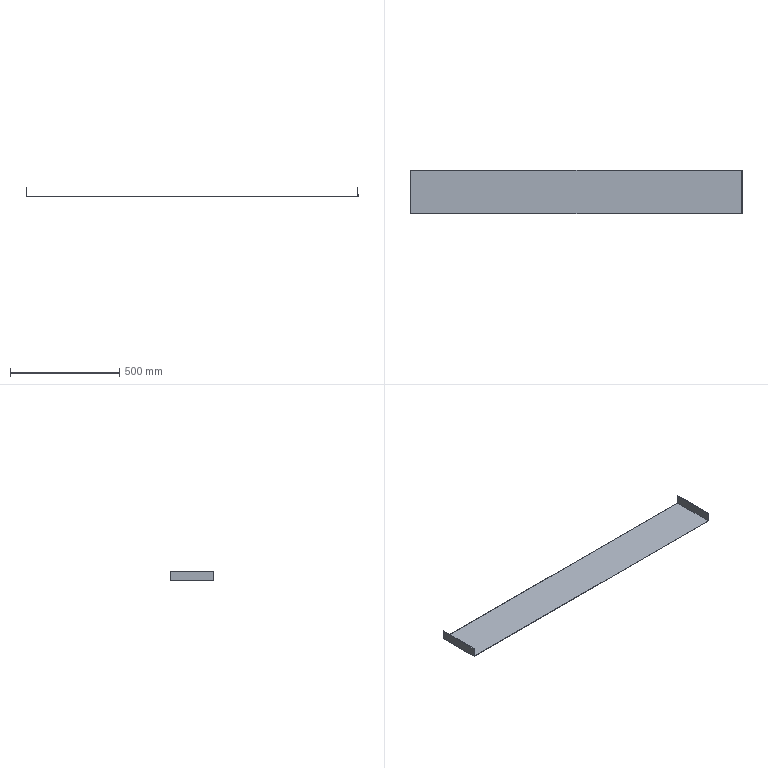Part | SolidWorks | features Extrusion 1, ICE 1, MirrorPattern 1 | 1 solid | 10 faces | box 1518 x 200 x 41 mm | volume 351600 mm3 | plane 10
STEP:
#1=CARTESIAN_POINT('',(-756.,-100.,1.));
#2=VERTEX_POINT('',#1);
#3=CARTESIAN_POINT('',(756.,-100.,1.));
#4=VERTEX_POINT('',#3);
#5=CARTESIAN_POINT('',(-759.,-100.,1.));
#6=DIRECTION('',(1.,0.,0.));
#7=VECTOR('',#6,1000.);
#8=LINE('',#5,#7);
#9=EDGE_CURVE('',#2,#4,#8,.T.);
#10=ORIENTED_EDGE('',*,*,#9,.T.);
#11=CARTESIAN_POINT('',(756.,100.,1.));
#12=VERTEX_POINT('',#11);
#13=CARTESIAN_POINT('',(756.,100.,1.));
#14=DIRECTION('',(0.,1.,0.));
#15=VECTOR('',#14,1000.);
#16=LINE('',#13,#15);
#17=EDGE_CURVE('',#4,#12,#16,.T.);
#18=ORIENTED_EDGE('',*,*,#17,.T.);
#19=CARTESIAN_POINT('',(-756.,100.,1.));
#20=VERTEX_POINT('',#19);
#21=CARTESIAN_POINT('',(-759.,100.,1.));
#22=DIRECTION('',(-1.,0.,0.));
#23=VECTOR('',#22,1000.);
#24=LINE('',#21,#23);
#25=EDGE_CURVE('',#12,#20,#24,.T.);
#26=ORIENTED_EDGE('',*,*,#25,.T.);
#27=CARTESIAN_POINT('',(-756.,100.,1.));
#28=DIRECTION('',(0.,1.,0.));
#29=VECTOR('',#28,1000.);
#30=LINE('',#27,#29);
#31=EDGE_CURVE('',#2,#20,#30,.T.);
#32=ORIENTED_EDGE('',*,*,#31,.F.);
#33=EDGE_LOOP('',(#10,#18,#26,#32));
#34=FACE_OUTER_BOUND('',#33,.T.);
#35=CARTESIAN_POINT('',(0.,0.,1.));
#36=DIRECTION('',(0.,0.,-1.));
#37=DIRECTION('',(-1.,0.,0.));
#38=AXIS2_PLACEMENT_3D('',#35,#36,#37);
#39=PLANE('',#38);
#40=ADVANCED_FACE('',(#34),#39,.F.);
#41=CARTESIAN_POINT('',(759.,-100.,0.));
#42=VERTEX_POINT('',#41);
#43=CARTESIAN_POINT('',(759.,100.,0.));
#44=VERTEX_POINT('',#43);
#45=CARTESIAN_POINT('',(759.,-100.,0.));
#46=DIRECTION('',(0.,1.,0.));
#47=VECTOR('',#46,1000.);
#48=LINE('',#45,#47);
#49=EDGE_CURVE('',#42,#44,#48,.T.);
#50=ORIENTED_EDGE('',*,*,#49,.T.);
#51=CARTESIAN_POINT('',(759.,100.,41.));
#52=VERTEX_POINT('',#51);
#53=CARTESIAN_POINT('',(759.,100.,1.));
#54=DIRECTION('',(0.,0.,-1.));
#55=VECTOR('',#54,1000.);
#56=LINE('',#53,#55);
#57=EDGE_CURVE('',#52,#44,#56,.T.);
#58=ORIENTED_EDGE('',*,*,#57,.F.);
#59=CARTESIAN_POINT('',(759.,-100.,41.));
#60=VERTEX_POINT('',#59);
#61=CARTESIAN_POINT('',(759.,100.,41.));
#62=DIRECTION('',(0.,-1.,0.));
#63=VECTOR('',#62,1000.);
#64=LINE('',#61,#63);
#65=EDGE_CURVE('',#52,#60,#64,.T.);
#66=ORIENTED_EDGE('',*,*,#65,.T.);
#67=CARTESIAN_POINT('',(759.,-100.,1.));
#68=DIRECTION('',(0.,0.,-1.));
#69=VECTOR('',#68,1000.);
#70=LINE('',#67,#69);
#71=EDGE_CURVE('',#60,#42,#70,.T.);
#72=ORIENTED_EDGE('',*,*,#71,.T.);
#73=EDGE_LOOP('',(#50,#58,#66,#72));
#74=FACE_OUTER_BOUND('',#73,.T.);
#75=CARTESIAN_POINT('',(759.,-100.,1.));
#76=DIRECTION('',(-1.,0.,0.));
#77=DIRECTION('',(0.,0.,1.));
#78=AXIS2_PLACEMENT_3D('',#75,#76,#77);
#79=PLANE('',#78);
#80=ADVANCED_FACE('',(#74),#79,.F.);
#81=CARTESIAN_POINT('',(-759.,100.,0.));
#82=VERTEX_POINT('',#81);
#83=CARTESIAN_POINT('',(-759.,100.,0.));
#84=DIRECTION('',(-1.,0.,0.));
#85=VECTOR('',#84,1000.);
#86=LINE('',#83,#85);
#87=EDGE_CURVE('',#44,#82,#86,.T.);
#88=ORIENTED_EDGE('',*,*,#87,.T.);
#89=CARTESIAN_POINT('',(-759.,100.,41.));
#90=VERTEX_POINT('',#89);
#91=CARTESIAN_POINT('',(-759.,100.,1.));
#92=DIRECTION('',(0.,0.,-1.));
#93=VECTOR('',#92,1000.);
#94=LINE('',#91,#93);
#95=EDGE_CURVE('',#90,#82,#94,.T.);
#96=ORIENTED_EDGE('',*,*,#95,.F.);
#97=CARTESIAN_POINT('',(-756.,100.,41.));
#98=VERTEX_POINT('',#97);
#99=CARTESIAN_POINT('',(-759.,100.,41.));
#100=DIRECTION('',(-1.,0.,0.));
#101=VECTOR('',#100,1000.);
#102=LINE('',#99,#101);
#103=EDGE_CURVE('',#98,#90,#102,.T.);
#104=ORIENTED_EDGE('',*,*,#103,.F.);
#105=CARTESIAN_POINT('',(-756.,100.,41.));
#106=DIRECTION('',(0.,0.,-1.));
#107=VECTOR('',#106,1000.);
#108=LINE('',#105,#107);
#109=EDGE_CURVE('',#98,#20,#108,.T.);
#110=ORIENTED_EDGE('',*,*,#109,.T.);
#111=ORIENTED_EDGE('',*,*,#25,.F.);
#112=CARTESIAN_POINT('',(756.,100.,41.));
#113=VERTEX_POINT('',#112);
#114=CARTESIAN_POINT('',(756.,100.,41.));
#115=DIRECTION('',(0.,0.,-1.));
#116=VECTOR('',#115,1000.);
#117=LINE('',#114,#116);
#118=EDGE_CURVE('',#113,#12,#117,.T.);
#119=ORIENTED_EDGE('',*,*,#118,.F.);
#120=CARTESIAN_POINT('',(759.,100.,41.));
#121=DIRECTION('',(1.,0.,0.));
#122=VECTOR('',#121,1000.);
#123=LINE('',#120,#122);
#124=EDGE_CURVE('',#113,#52,#123,.T.);
#125=ORIENTED_EDGE('',*,*,#124,.T.);
#126=ORIENTED_EDGE('',*,*,#57,.T.);
#127=EDGE_LOOP('',(#88,#96,#104,#110,#111,#119,#125,#126));
#128=FACE_OUTER_BOUND('',#127,.T.);
#129=CARTESIAN_POINT('',(-759.,100.,1.));
#130=DIRECTION('',(0.,-1.,0.));
#131=DIRECTION('',(0.,0.,-1.));
#132=AXIS2_PLACEMENT_3D('',#129,#130,#131);
#133=PLANE('',#132);
#134=ADVANCED_FACE('',(#128),#133,.F.);
#135=CARTESIAN_POINT('',(-759.,-100.,0.));
#136=VERTEX_POINT('',#135);
#137=CARTESIAN_POINT('',(-759.,-100.,0.));
#138=DIRECTION('',(0.,-1.,0.));
#139=VECTOR('',#138,1000.);
#140=LINE('',#137,#139);
#141=EDGE_CURVE('',#82,#136,#140,.T.);
#142=ORIENTED_EDGE('',*,*,#141,.T.);
#143=CARTESIAN_POINT('',(-759.,-100.,41.));
#144=VERTEX_POINT('',#143);
#145=CARTESIAN_POINT('',(-759.,-100.,1.));
#146=DIRECTION('',(0.,0.,-1.));
#147=VECTOR('',#146,1000.);
#148=LINE('',#145,#147);
#149=EDGE_CURVE('',#144,#136,#148,.T.);
#150=ORIENTED_EDGE('',*,*,#149,.F.);
#151=CARTESIAN_POINT('',(-759.,100.,41.));
#152=DIRECTION('',(0.,-1.,0.));
#153=VECTOR('',#152,1000.);
#154=LINE('',#151,#153);
#155=EDGE_CURVE('',#90,#144,#154,.T.);
#156=ORIENTED_EDGE('',*,*,#155,.F.);
#157=ORIENTED_EDGE('',*,*,#95,.T.);
#158=EDGE_LOOP('',(#142,#150,#156,#157));
#159=FACE_OUTER_BOUND('',#158,.T.);
#160=CARTESIAN_POINT('',(-759.,-100.,1.));
#161=DIRECTION('',(1.,0.,0.));
#162=DIRECTION('',(0.,0.,-1.));
#163=AXIS2_PLACEMENT_3D('',#160,#161,#162);
#164=PLANE('',#163);
#165=ADVANCED_FACE('',(#159),#164,.F.);
#166=CARTESIAN_POINT('',(-759.,-100.,0.));
#167=DIRECTION('',(1.,0.,0.));
#168=VECTOR('',#167,1000.);
#169=LINE('',#166,#168);
#170=EDGE_CURVE('',#136,#42,#169,.T.);
#171=ORIENTED_EDGE('',*,*,#170,.T.);
#172=ORIENTED_EDGE('',*,*,#71,.F.);
#173=CARTESIAN_POINT('',(756.,-100.,41.));
#174=VERTEX_POINT('',#173);
#175=CARTESIAN_POINT('',(759.,-100.,41.));
#176=DIRECTION('',(-1.,0.,0.));
#177=VECTOR('',#176,1000.);
#178=LINE('',#175,#177);
#179=EDGE_CURVE('',#60,#174,#178,.T.);
#180=ORIENTED_EDGE('',*,*,#179,.T.);
#181=CARTESIAN_POINT('',(756.,-100.,41.));
#182=DIRECTION('',(0.,0.,-1.));
#183=VECTOR('',#182,1000.);
#184=LINE('',#181,#183);
#185=EDGE_CURVE('',#174,#4,#184,.T.);
#186=ORIENTED_EDGE('',*,*,#185,.T.);
#187=ORIENTED_EDGE('',*,*,#9,.F.);
#188=CARTESIAN_POINT('',(-756.,-100.,41.));
#189=VERTEX_POINT('',#188);
#190=CARTESIAN_POINT('',(-756.,-100.,41.));
#191=DIRECTION('',(0.,0.,-1.));
#192=VECTOR('',#191,1000.);
#193=LINE('',#190,#192);
#194=EDGE_CURVE('',#189,#2,#193,.T.);
#195=ORIENTED_EDGE('',*,*,#194,.F.);
#196=CARTESIAN_POINT('',(-759.,-100.,41.));
#197=DIRECTION('',(1.,0.,0.));
#198=VECTOR('',#197,1000.);
#199=LINE('',#196,#198);
#200=EDGE_CURVE('',#144,#189,#199,.T.);
#201=ORIENTED_EDGE('',*,*,#200,.F.);
#202=ORIENTED_EDGE('',*,*,#149,.T.);
#203=EDGE_LOOP('',(#171,#172,#180,#186,#187,#195,#201,#202));
#204=FACE_OUTER_BOUND('',#203,.T.);
#205=CARTESIAN_POINT('',(-759.,-100.,1.));
#206=DIRECTION('',(0.,1.,0.));
#207=DIRECTION('',(0.,0.,1.));
#208=AXIS2_PLACEMENT_3D('',#205,#206,#207);
#209=PLANE('',#208);
#210=ADVANCED_FACE('',(#204),#209,.F.);
#211=ORIENTED_EDGE('',*,*,#49,.F.);
#212=ORIENTED_EDGE('',*,*,#170,.F.);
#213=ORIENTED_EDGE('',*,*,#141,.F.);
#214=ORIENTED_EDGE('',*,*,#87,.F.);
#215=EDGE_LOOP('',(#211,#212,#213,#214));
#216=FACE_OUTER_BOUND('',#215,.T.);
#217=CARTESIAN_POINT('',(0.,0.,0.));
#218=DIRECTION('',(0.,0.,-1.));
#219=DIRECTION('',(-1.,0.,0.));
#220=AXIS2_PLACEMENT_3D('',#217,#218,#219);
#221=PLANE('',#220);
#222=ADVANCED_FACE('',(#216),#221,.T.);
#223=ORIENTED_EDGE('',*,*,#31,.T.);
#224=ORIENTED_EDGE('',*,*,#109,.F.);
#225=CARTESIAN_POINT('',(-756.,100.,41.));
#226=DIRECTION('',(0.,1.,0.));
#227=VECTOR('',#226,1000.);
#228=LINE('',#225,#227);
#229=EDGE_CURVE('',#189,#98,#228,.T.);
#230=ORIENTED_EDGE('',*,*,#229,.F.);
#231=ORIENTED_EDGE('',*,*,#194,.T.);
#232=EDGE_LOOP('',(#223,#224,#230,#231));
#233=FACE_OUTER_BOUND('',#232,.T.);
#234=CARTESIAN_POINT('',(-756.,100.,41.));
#235=DIRECTION('',(-1.,0.,0.));
#236=DIRECTION('',(0.,0.,1.));
#237=AXIS2_PLACEMENT_3D('',#234,#235,#236);
#238=PLANE('',#237);
#239=ADVANCED_FACE('',(#233),#238,.F.);
#240=ORIENTED_EDGE('',*,*,#155,.T.);
#241=ORIENTED_EDGE('',*,*,#200,.T.);
#242=ORIENTED_EDGE('',*,*,#229,.T.);
#243=ORIENTED_EDGE('',*,*,#103,.T.);
#244=EDGE_LOOP('',(#240,#241,#242,#243));
#245=FACE_OUTER_BOUND('',#244,.T.);
#246=CARTESIAN_POINT('',(0.,0.,41.));
#247=DIRECTION('',(0.,0.,1.));
#248=DIRECTION('',(1.,0.,0.));
#249=AXIS2_PLACEMENT_3D('',#246,#247,#248);
#250=PLANE('',#249);
#251=ADVANCED_FACE('',(#245),#250,.T.);
#252=ORIENTED_EDGE('',*,*,#17,.F.);
#253=ORIENTED_EDGE('',*,*,#185,.F.);
#254=CARTESIAN_POINT('',(756.,100.,41.));
#255=DIRECTION('',(0.,1.,0.));
#256=VECTOR('',#255,1000.);
#257=LINE('',#254,#256);
#258=EDGE_CURVE('',#174,#113,#257,.T.);
#259=ORIENTED_EDGE('',*,*,#258,.T.);
#260=ORIENTED_EDGE('',*,*,#118,.T.);
#261=EDGE_LOOP('',(#252,#253,#259,#260));
#262=FACE_OUTER_BOUND('',#261,.T.);
#263=CARTESIAN_POINT('',(756.,100.,41.));
#264=DIRECTION('',(-1.,0.,0.));
#265=DIRECTION('',(0.,0.,1.));
#266=AXIS2_PLACEMENT_3D('',#263,#264,#265);
#267=PLANE('',#266);
#268=ADVANCED_FACE('',(#262),#267,.T.);
#269=ORIENTED_EDGE('',*,*,#65,.F.);
#270=ORIENTED_EDGE('',*,*,#124,.F.);
#271=ORIENTED_EDGE('',*,*,#258,.F.);
#272=ORIENTED_EDGE('',*,*,#179,.F.);
#273=EDGE_LOOP('',(#269,#270,#271,#272));
#274=FACE_OUTER_BOUND('',#273,.T.);
#275=CARTESIAN_POINT('',(0.,0.,41.));
#276=DIRECTION('',(0.,0.,1.));
#277=DIRECTION('',(-1.,0.,0.));
#278=AXIS2_PLACEMENT_3D('',#275,#276,#277);
#279=PLANE('',#278);
#280=ADVANCED_FACE('',(#274),#279,.T.);
#281=CLOSED_SHELL('',(#40,#80,#134,#165,#210,#222,#239,#251,#268,#280));
#282=MANIFOLD_SOLID_BREP('',#281);
#283=CARTESIAN_POINT('',(0.,0.,0.));
#284=DIRECTION('',(0.,0.,1.));
#285=DIRECTION('',(1.,0.,0.));
#286=AXIS2_PLACEMENT_3D('',#283,#284,#285);
#287=(LENGTH_UNIT()NAMED_UNIT(*)SI_UNIT(.MILLI.,.METRE.));
#288=UNCERTAINTY_MEASURE_WITH_UNIT(LENGTH_MEASURE(0.00001),#287,'','');
#289=(NAMED_UNIT(*)PLANE_ANGLE_UNIT()SI_UNIT($,.RADIAN.));
#290=(NAMED_UNIT(*)SI_UNIT($,.STERADIAN.)SOLID_ANGLE_UNIT());
#291=(GEOMETRIC_REPRESENTATION_CONTEXT(3)GLOBAL_UNCERTAINTY_ASSIGNED_CONTEXT((#288))GLOBAL_UNIT_ASSIGNED_CONTEXT((#287,#289,#290))REPRESENTATION_CONTEXT('',''));
#292=ADVANCED_BREP_SHAPE_REPRESENTATION('',(#282,#286),#291);